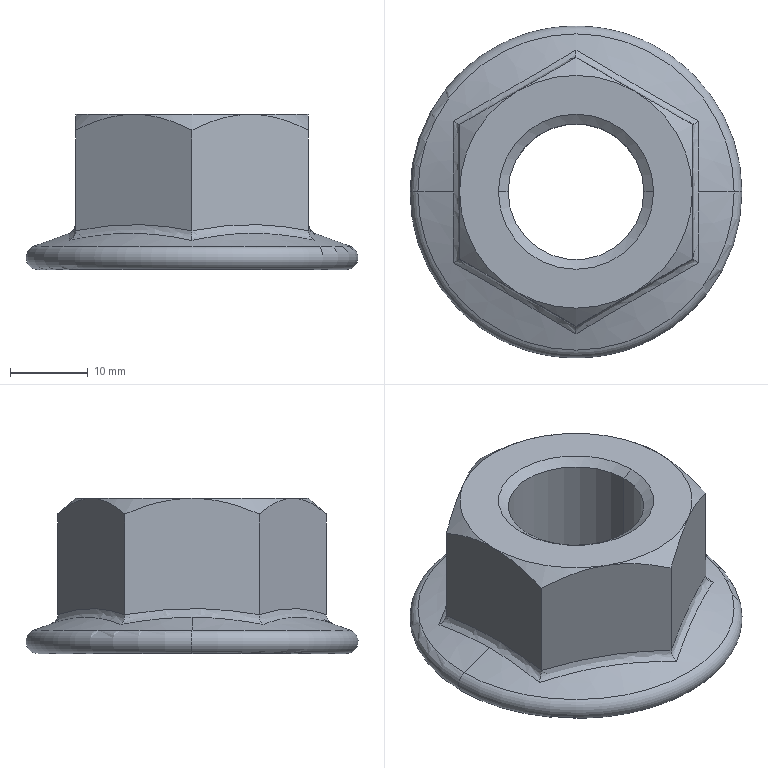Part | STEP file | hex flange nut_am_B18.2.2.4M - Hex flange nut, M20 x 2.5 --N | 1 solid | 32 faces | box 42.8 x 42.8 x 20 mm | volume 12973 mm3 | cone 12 | plane 8 | spline 6 | cylinder 4 | torus 2 | commonest cylinder face diameters 17.5 x2 20 x2